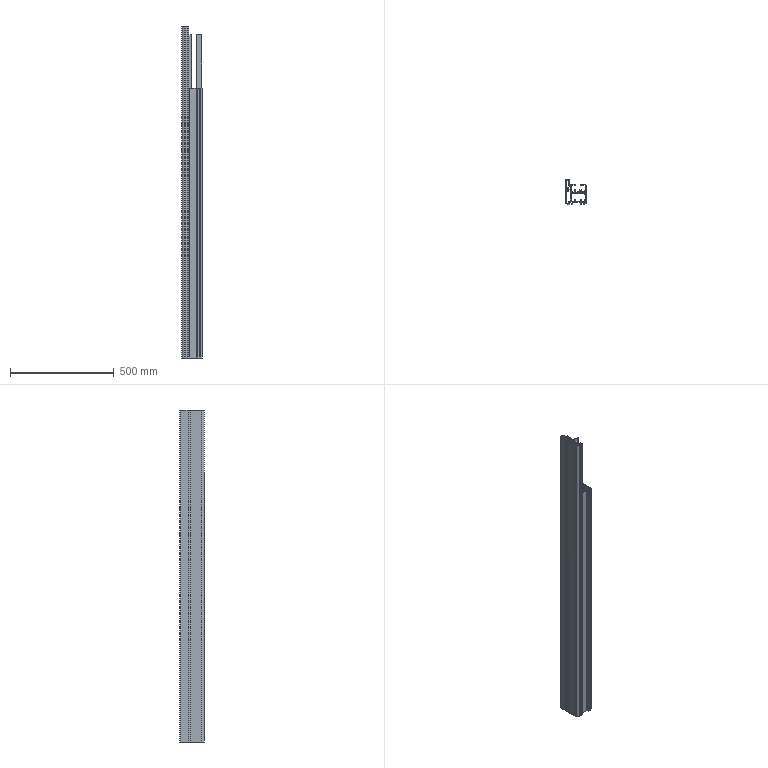Part | STEP file | 1 solid | 214 faces | box 100 x 118 x 1600 mm | volume 2600704 mm3 | plane 128 | cylinder 86 | commonest cylinder face diameters 1 x56 4 x22 24 x3 2 x2 10 x1 16 x1